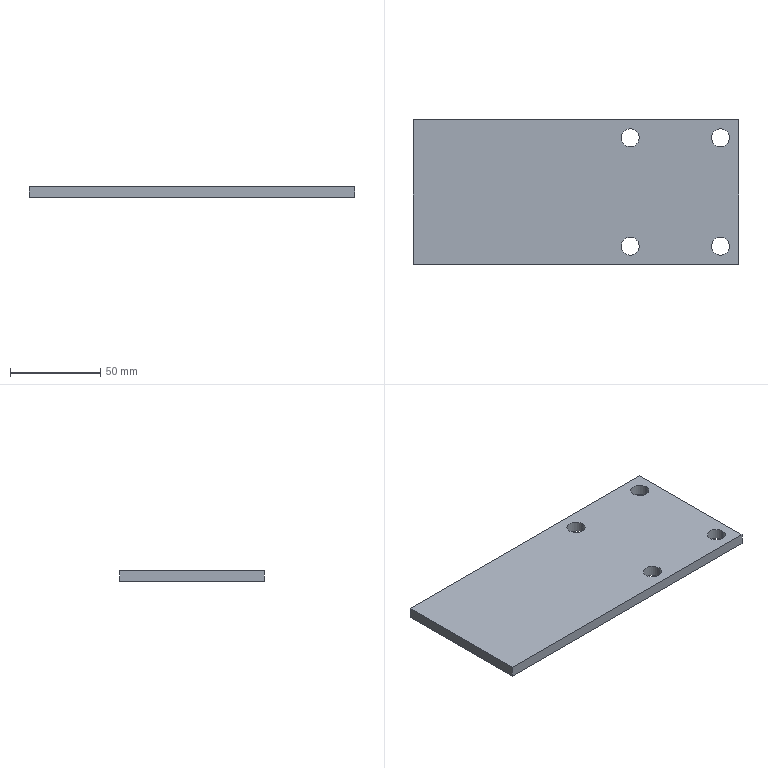Part | SolidWorks | features Extrusion 1, ICE 1 | 1 solid | 14 faces | box 180 x 80 x 6 mm | volume 84515 mm3 | cylinder 8 | plane 6 | commonest cylinder face diameters 10 x8
STEP:
#1=CARTESIAN_POINT('',(165.,9.999,0.));
#2=VERTEX_POINT('',#1);
#3=CARTESIAN_POINT('',(175.,9.999,0.));
#4=VERTEX_POINT('',#3);
#5=CARTESIAN_POINT('',(170.,9.999,0.));
#6=DIRECTION('',(0.,0.,1.));
#7=DIRECTION('',(1.,0.,0.));
#8=AXIS2_PLACEMENT_3D('',#5,#6,#7);
#9=CIRCLE('',#8,5.);
#10=EDGE_CURVE('',#2,#4,#9,.T.);
#11=ORIENTED_EDGE('',*,*,#10,.F.);
#12=CARTESIAN_POINT('',(165.,9.999,6.));
#13=VERTEX_POINT('',#12);
#14=CARTESIAN_POINT('',(165.,9.999,0.));
#15=DIRECTION('',(0.,0.,1.));
#16=VECTOR('',#15,1000.);
#17=LINE('',#14,#16);
#18=EDGE_CURVE('',#2,#13,#17,.T.);
#19=ORIENTED_EDGE('',*,*,#18,.T.);
#20=CARTESIAN_POINT('',(175.,9.999,6.));
#21=VERTEX_POINT('',#20);
#22=CARTESIAN_POINT('',(170.,9.999,6.));
#23=DIRECTION('',(0.,0.,1.));
#24=DIRECTION('',(1.,0.,0.));
#25=AXIS2_PLACEMENT_3D('',#22,#23,#24);
#26=CIRCLE('',#25,5.);
#27=EDGE_CURVE('',#13,#21,#26,.T.);
#28=ORIENTED_EDGE('',*,*,#27,.T.);
#29=CARTESIAN_POINT('',(175.,9.999,0.));
#30=DIRECTION('',(0.,0.,1.));
#31=VECTOR('',#30,1000.);
#32=LINE('',#29,#31);
#33=EDGE_CURVE('',#4,#21,#32,.T.);
#34=ORIENTED_EDGE('',*,*,#33,.F.);
#35=EDGE_LOOP('',(#11,#19,#28,#34));
#36=FACE_OUTER_BOUND('',#35,.T.);
#37=CARTESIAN_POINT('',(170.,9.999,0.));
#38=DIRECTION('',(0.,0.,1.));
#39=DIRECTION('',(1.,0.,0.));
#40=AXIS2_PLACEMENT_3D('',#37,#38,#39);
#41=CYLINDRICAL_SURFACE('',#40,5.);
#42=ADVANCED_FACE('',(#36),#41,.F.);
#43=CARTESIAN_POINT('',(115.,9.999,0.));
#44=VERTEX_POINT('',#43);
#45=CARTESIAN_POINT('',(125.,9.999,0.));
#46=VERTEX_POINT('',#45);
#47=CARTESIAN_POINT('',(120.,9.999,0.));
#48=DIRECTION('',(0.,0.,1.));
#49=DIRECTION('',(1.,0.,0.));
#50=AXIS2_PLACEMENT_3D('',#47,#48,#49);
#51=CIRCLE('',#50,5.);
#52=EDGE_CURVE('',#44,#46,#51,.T.);
#53=ORIENTED_EDGE('',*,*,#52,.F.);
#54=CARTESIAN_POINT('',(115.,9.999,6.));
#55=VERTEX_POINT('',#54);
#56=CARTESIAN_POINT('',(115.,9.999,0.));
#57=DIRECTION('',(0.,0.,1.));
#58=VECTOR('',#57,1000.);
#59=LINE('',#56,#58);
#60=EDGE_CURVE('',#44,#55,#59,.T.);
#61=ORIENTED_EDGE('',*,*,#60,.T.);
#62=CARTESIAN_POINT('',(125.,9.999,6.));
#63=VERTEX_POINT('',#62);
#64=CARTESIAN_POINT('',(120.,9.999,6.));
#65=DIRECTION('',(0.,0.,1.));
#66=DIRECTION('',(1.,0.,0.));
#67=AXIS2_PLACEMENT_3D('',#64,#65,#66);
#68=CIRCLE('',#67,5.);
#69=EDGE_CURVE('',#55,#63,#68,.T.);
#70=ORIENTED_EDGE('',*,*,#69,.T.);
#71=CARTESIAN_POINT('',(125.,9.999,0.));
#72=DIRECTION('',(0.,0.,1.));
#73=VECTOR('',#72,1000.);
#74=LINE('',#71,#73);
#75=EDGE_CURVE('',#46,#63,#74,.T.);
#76=ORIENTED_EDGE('',*,*,#75,.F.);
#77=EDGE_LOOP('',(#53,#61,#70,#76));
#78=FACE_OUTER_BOUND('',#77,.T.);
#79=CARTESIAN_POINT('',(120.,9.999,0.));
#80=DIRECTION('',(0.,0.,1.));
#81=DIRECTION('',(1.,0.,0.));
#82=AXIS2_PLACEMENT_3D('',#79,#80,#81);
#83=CYLINDRICAL_SURFACE('',#82,5.);
#84=ADVANCED_FACE('',(#78),#83,.F.);
#85=CARTESIAN_POINT('',(115.,69.999,0.));
#86=VERTEX_POINT('',#85);
#87=CARTESIAN_POINT('',(125.,69.999,0.));
#88=VERTEX_POINT('',#87);
#89=CARTESIAN_POINT('',(120.,69.999,0.));
#90=DIRECTION('',(0.,0.,1.));
#91=DIRECTION('',(1.,0.,0.));
#92=AXIS2_PLACEMENT_3D('',#89,#90,#91);
#93=CIRCLE('',#92,5.);
#94=EDGE_CURVE('',#86,#88,#93,.T.);
#95=ORIENTED_EDGE('',*,*,#94,.F.);
#96=CARTESIAN_POINT('',(115.,69.999,6.));
#97=VERTEX_POINT('',#96);
#98=CARTESIAN_POINT('',(115.,69.999,0.));
#99=DIRECTION('',(0.,0.,1.));
#100=VECTOR('',#99,1000.);
#101=LINE('',#98,#100);
#102=EDGE_CURVE('',#86,#97,#101,.T.);
#103=ORIENTED_EDGE('',*,*,#102,.T.);
#104=CARTESIAN_POINT('',(125.,69.999,6.));
#105=VERTEX_POINT('',#104);
#106=CARTESIAN_POINT('',(120.,69.999,6.));
#107=DIRECTION('',(0.,0.,1.));
#108=DIRECTION('',(1.,0.,0.));
#109=AXIS2_PLACEMENT_3D('',#106,#107,#108);
#110=CIRCLE('',#109,5.);
#111=EDGE_CURVE('',#97,#105,#110,.T.);
#112=ORIENTED_EDGE('',*,*,#111,.T.);
#113=CARTESIAN_POINT('',(125.,69.999,0.));
#114=DIRECTION('',(0.,0.,1.));
#115=VECTOR('',#114,1000.);
#116=LINE('',#113,#115);
#117=EDGE_CURVE('',#88,#105,#116,.T.);
#118=ORIENTED_EDGE('',*,*,#117,.F.);
#119=EDGE_LOOP('',(#95,#103,#112,#118));
#120=FACE_OUTER_BOUND('',#119,.T.);
#121=CARTESIAN_POINT('',(120.,69.999,0.));
#122=DIRECTION('',(0.,0.,1.));
#123=DIRECTION('',(1.,0.,0.));
#124=AXIS2_PLACEMENT_3D('',#121,#122,#123);
#125=CYLINDRICAL_SURFACE('',#124,5.);
#126=ADVANCED_FACE('',(#120),#125,.F.);
#127=CARTESIAN_POINT('',(165.,69.999,0.));
#128=VERTEX_POINT('',#127);
#129=CARTESIAN_POINT('',(175.,69.999,0.));
#130=VERTEX_POINT('',#129);
#131=CARTESIAN_POINT('',(170.,69.999,0.));
#132=DIRECTION('',(0.,0.,1.));
#133=DIRECTION('',(1.,0.,0.));
#134=AXIS2_PLACEMENT_3D('',#131,#132,#133);
#135=CIRCLE('',#134,5.);
#136=EDGE_CURVE('',#128,#130,#135,.T.);
#137=ORIENTED_EDGE('',*,*,#136,.F.);
#138=CARTESIAN_POINT('',(165.,69.999,6.));
#139=VERTEX_POINT('',#138);
#140=CARTESIAN_POINT('',(165.,69.999,0.));
#141=DIRECTION('',(0.,0.,1.));
#142=VECTOR('',#141,1000.);
#143=LINE('',#140,#142);
#144=EDGE_CURVE('',#128,#139,#143,.T.);
#145=ORIENTED_EDGE('',*,*,#144,.T.);
#146=CARTESIAN_POINT('',(175.,69.999,6.));
#147=VERTEX_POINT('',#146);
#148=CARTESIAN_POINT('',(170.,69.999,6.));
#149=DIRECTION('',(0.,0.,1.));
#150=DIRECTION('',(1.,0.,0.));
#151=AXIS2_PLACEMENT_3D('',#148,#149,#150);
#152=CIRCLE('',#151,5.);
#153=EDGE_CURVE('',#139,#147,#152,.T.);
#154=ORIENTED_EDGE('',*,*,#153,.T.);
#155=CARTESIAN_POINT('',(175.,69.999,0.));
#156=DIRECTION('',(0.,0.,1.));
#157=VECTOR('',#156,1000.);
#158=LINE('',#155,#157);
#159=EDGE_CURVE('',#130,#147,#158,.T.);
#160=ORIENTED_EDGE('',*,*,#159,.F.);
#161=EDGE_LOOP('',(#137,#145,#154,#160));
#162=FACE_OUTER_BOUND('',#161,.T.);
#163=CARTESIAN_POINT('',(170.,69.999,0.));
#164=DIRECTION('',(0.,0.,1.));
#165=DIRECTION('',(1.,0.,0.));
#166=AXIS2_PLACEMENT_3D('',#163,#164,#165);
#167=CYLINDRICAL_SURFACE('',#166,5.);
#168=ADVANCED_FACE('',(#162),#167,.F.);
#169=CARTESIAN_POINT('',(0.,0.,0.));
#170=VERTEX_POINT('',#169);
#171=CARTESIAN_POINT('',(180.,0.,0.));
#172=VERTEX_POINT('',#171);
#173=CARTESIAN_POINT('',(180.,0.,0.));
#174=DIRECTION('',(1.,0.,0.));
#175=VECTOR('',#174,1000.);
#176=LINE('',#173,#175);
#177=EDGE_CURVE('',#170,#172,#176,.T.);
#178=ORIENTED_EDGE('',*,*,#177,.T.);
#179=CARTESIAN_POINT('',(180.,0.,6.));
#180=VERTEX_POINT('',#179);
#181=CARTESIAN_POINT('',(180.,0.,6.));
#182=DIRECTION('',(0.,0.,-1.));
#183=VECTOR('',#182,1000.);
#184=LINE('',#181,#183);
#185=EDGE_CURVE('',#180,#172,#184,.T.);
#186=ORIENTED_EDGE('',*,*,#185,.F.);
#187=CARTESIAN_POINT('',(0.,0.,6.));
#188=VERTEX_POINT('',#187);
#189=CARTESIAN_POINT('',(180.,0.,6.));
#190=DIRECTION('',(1.,0.,0.));
#191=VECTOR('',#190,1000.);
#192=LINE('',#189,#191);
#193=EDGE_CURVE('',#188,#180,#192,.T.);
#194=ORIENTED_EDGE('',*,*,#193,.F.);
#195=CARTESIAN_POINT('',(0.,0.,6.));
#196=DIRECTION('',(0.,0.,-1.));
#197=VECTOR('',#196,1000.);
#198=LINE('',#195,#197);
#199=EDGE_CURVE('',#188,#170,#198,.T.);
#200=ORIENTED_EDGE('',*,*,#199,.T.);
#201=EDGE_LOOP('',(#178,#186,#194,#200));
#202=FACE_OUTER_BOUND('',#201,.T.);
#203=CARTESIAN_POINT('',(180.,0.,6.));
#204=DIRECTION('',(0.,1.,0.));
#205=DIRECTION('',(0.,0.,1.));
#206=AXIS2_PLACEMENT_3D('',#203,#204,#205);
#207=PLANE('',#206);
#208=ADVANCED_FACE('',(#202),#207,.F.);
#209=CARTESIAN_POINT('',(180.,80.,0.));
#210=VERTEX_POINT('',#209);
#211=CARTESIAN_POINT('',(180.,80.,0.));
#212=DIRECTION('',(0.,1.,0.));
#213=VECTOR('',#212,1000.);
#214=LINE('',#211,#213);
#215=EDGE_CURVE('',#172,#210,#214,.T.);
#216=ORIENTED_EDGE('',*,*,#215,.T.);
#217=CARTESIAN_POINT('',(180.,80.,6.));
#218=VERTEX_POINT('',#217);
#219=CARTESIAN_POINT('',(180.,80.,6.));
#220=DIRECTION('',(0.,0.,-1.));
#221=VECTOR('',#220,1000.);
#222=LINE('',#219,#221);
#223=EDGE_CURVE('',#218,#210,#222,.T.);
#224=ORIENTED_EDGE('',*,*,#223,.F.);
#225=CARTESIAN_POINT('',(180.,80.,6.));
#226=DIRECTION('',(0.,1.,0.));
#227=VECTOR('',#226,1000.);
#228=LINE('',#225,#227);
#229=EDGE_CURVE('',#180,#218,#228,.T.);
#230=ORIENTED_EDGE('',*,*,#229,.F.);
#231=ORIENTED_EDGE('',*,*,#185,.T.);
#232=EDGE_LOOP('',(#216,#224,#230,#231));
#233=FACE_OUTER_BOUND('',#232,.T.);
#234=CARTESIAN_POINT('',(180.,80.,6.));
#235=DIRECTION('',(-1.,0.,0.));
#236=DIRECTION('',(0.,0.,1.));
#237=AXIS2_PLACEMENT_3D('',#234,#235,#236);
#238=PLANE('',#237);
#239=ADVANCED_FACE('',(#233),#238,.F.);
#240=CARTESIAN_POINT('',(0.,80.,0.));
#241=VERTEX_POINT('',#240);
#242=CARTESIAN_POINT('',(0.,80.,0.));
#243=DIRECTION('',(-1.,0.,0.));
#244=VECTOR('',#243,1000.);
#245=LINE('',#242,#244);
#246=EDGE_CURVE('',#210,#241,#245,.T.);
#247=ORIENTED_EDGE('',*,*,#246,.T.);
#248=CARTESIAN_POINT('',(0.,80.,6.));
#249=VERTEX_POINT('',#248);
#250=CARTESIAN_POINT('',(0.,80.,6.));
#251=DIRECTION('',(0.,0.,-1.));
#252=VECTOR('',#251,1000.);
#253=LINE('',#250,#252);
#254=EDGE_CURVE('',#249,#241,#253,.T.);
#255=ORIENTED_EDGE('',*,*,#254,.F.);
#256=CARTESIAN_POINT('',(0.,80.,6.));
#257=DIRECTION('',(-1.,0.,0.));
#258=VECTOR('',#257,1000.);
#259=LINE('',#256,#258);
#260=EDGE_CURVE('',#218,#249,#259,.T.);
#261=ORIENTED_EDGE('',*,*,#260,.F.);
#262=ORIENTED_EDGE('',*,*,#223,.T.);
#263=EDGE_LOOP('',(#247,#255,#261,#262));
#264=FACE_OUTER_BOUND('',#263,.T.);
#265=CARTESIAN_POINT('',(0.,80.,6.));
#266=DIRECTION('',(0.,-1.,0.));
#267=DIRECTION('',(0.,0.,-1.));
#268=AXIS2_PLACEMENT_3D('',#265,#266,#267);
#269=PLANE('',#268);
#270=ADVANCED_FACE('',(#264),#269,.F.);
#271=CARTESIAN_POINT('',(0.,0.,0.));
#272=DIRECTION('',(0.,-1.,0.));
#273=VECTOR('',#272,1000.);
#274=LINE('',#271,#273);
#275=EDGE_CURVE('',#241,#170,#274,.T.);
#276=ORIENTED_EDGE('',*,*,#275,.T.);
#277=ORIENTED_EDGE('',*,*,#199,.F.);
#278=CARTESIAN_POINT('',(0.,0.,6.));
#279=DIRECTION('',(0.,-1.,0.));
#280=VECTOR('',#279,1000.);
#281=LINE('',#278,#280);
#282=EDGE_CURVE('',#249,#188,#281,.T.);
#283=ORIENTED_EDGE('',*,*,#282,.F.);
#284=ORIENTED_EDGE('',*,*,#254,.T.);
#285=EDGE_LOOP('',(#276,#277,#283,#284));
#286=FACE_OUTER_BOUND('',#285,.T.);
#287=CARTESIAN_POINT('',(0.,0.,6.));
#288=DIRECTION('',(1.,0.,0.));
#289=DIRECTION('',(0.,0.,-1.));
#290=AXIS2_PLACEMENT_3D('',#287,#288,#289);
#291=PLANE('',#290);
#292=ADVANCED_FACE('',(#286),#291,.F.);
#293=CARTESIAN_POINT('',(170.,9.999,6.));
#294=DIRECTION('',(0.,0.,1.));
#295=DIRECTION('',(1.,0.,0.));
#296=AXIS2_PLACEMENT_3D('',#293,#294,#295);
#297=CIRCLE('',#296,5.);
#298=EDGE_CURVE('',#21,#13,#297,.T.);
#299=ORIENTED_EDGE('',*,*,#298,.F.);
#300=ORIENTED_EDGE('',*,*,#27,.F.);
#301=EDGE_LOOP('',(#299,#300));
#302=FACE_BOUND('',#301,.T.);
#303=CARTESIAN_POINT('',(120.,9.999,6.));
#304=DIRECTION('',(0.,0.,1.));
#305=DIRECTION('',(1.,0.,0.));
#306=AXIS2_PLACEMENT_3D('',#303,#304,#305);
#307=CIRCLE('',#306,5.);
#308=EDGE_CURVE('',#63,#55,#307,.T.);
#309=ORIENTED_EDGE('',*,*,#308,.F.);
#310=ORIENTED_EDGE('',*,*,#69,.F.);
#311=EDGE_LOOP('',(#309,#310));
#312=FACE_BOUND('',#311,.T.);
#313=CARTESIAN_POINT('',(120.,69.999,6.));
#314=DIRECTION('',(0.,0.,1.));
#315=DIRECTION('',(1.,0.,0.));
#316=AXIS2_PLACEMENT_3D('',#313,#314,#315);
#317=CIRCLE('',#316,5.);
#318=EDGE_CURVE('',#105,#97,#317,.T.);
#319=ORIENTED_EDGE('',*,*,#318,.F.);
#320=ORIENTED_EDGE('',*,*,#111,.F.);
#321=EDGE_LOOP('',(#319,#320));
#322=FACE_BOUND('',#321,.T.);
#323=CARTESIAN_POINT('',(170.,69.999,6.));
#324=DIRECTION('',(0.,0.,1.));
#325=DIRECTION('',(1.,0.,0.));
#326=AXIS2_PLACEMENT_3D('',#323,#324,#325);
#327=CIRCLE('',#326,5.);
#328=EDGE_CURVE('',#147,#139,#327,.T.);
#329=ORIENTED_EDGE('',*,*,#328,.F.);
#330=ORIENTED_EDGE('',*,*,#153,.F.);
#331=EDGE_LOOP('',(#329,#330));
#332=FACE_BOUND('',#331,.T.);
#333=ORIENTED_EDGE('',*,*,#193,.T.);
#334=ORIENTED_EDGE('',*,*,#229,.T.);
#335=ORIENTED_EDGE('',*,*,#260,.T.);
#336=ORIENTED_EDGE('',*,*,#282,.T.);
#337=EDGE_LOOP('',(#333,#334,#335,#336));
#338=FACE_OUTER_BOUND('',#337,.T.);
#339=CARTESIAN_POINT('',(0.,0.,6.));
#340=DIRECTION('',(0.,0.,-1.));
#341=DIRECTION('',(-1.,0.,0.));
#342=AXIS2_PLACEMENT_3D('',#339,#340,#341);
#343=PLANE('',#342);
#344=ADVANCED_FACE('',(#302,#312,#322,#332,#338),#343,.F.);
#345=CARTESIAN_POINT('',(170.,9.999,0.));
#346=DIRECTION('',(0.,0.,1.));
#347=DIRECTION('',(1.,0.,0.));
#348=AXIS2_PLACEMENT_3D('',#345,#346,#347);
#349=CIRCLE('',#348,5.);
#350=EDGE_CURVE('',#4,#2,#349,.T.);
#351=ORIENTED_EDGE('',*,*,#350,.T.);
#352=ORIENTED_EDGE('',*,*,#10,.T.);
#353=EDGE_LOOP('',(#351,#352));
#354=FACE_BOUND('',#353,.T.);
#355=CARTESIAN_POINT('',(120.,9.999,0.));
#356=DIRECTION('',(0.,0.,1.));
#357=DIRECTION('',(1.,0.,0.));
#358=AXIS2_PLACEMENT_3D('',#355,#356,#357);
#359=CIRCLE('',#358,5.);
#360=EDGE_CURVE('',#46,#44,#359,.T.);
#361=ORIENTED_EDGE('',*,*,#360,.T.);
#362=ORIENTED_EDGE('',*,*,#52,.T.);
#363=EDGE_LOOP('',(#361,#362));
#364=FACE_BOUND('',#363,.T.);
#365=CARTESIAN_POINT('',(120.,69.999,0.));
#366=DIRECTION('',(0.,0.,1.));
#367=DIRECTION('',(1.,0.,0.));
#368=AXIS2_PLACEMENT_3D('',#365,#366,#367);
#369=CIRCLE('',#368,5.);
#370=EDGE_CURVE('',#88,#86,#369,.T.);
#371=ORIENTED_EDGE('',*,*,#370,.T.);
#372=ORIENTED_EDGE('',*,*,#94,.T.);
#373=EDGE_LOOP('',(#371,#372));
#374=FACE_BOUND('',#373,.T.);
#375=CARTESIAN_POINT('',(170.,69.999,0.));
#376=DIRECTION('',(0.,0.,1.));
#377=DIRECTION('',(1.,0.,0.));
#378=AXIS2_PLACEMENT_3D('',#375,#376,#377);
#379=CIRCLE('',#378,5.);
#380=EDGE_CURVE('',#130,#128,#379,.T.);
#381=ORIENTED_EDGE('',*,*,#380,.T.);
#382=ORIENTED_EDGE('',*,*,#136,.T.);
#383=EDGE_LOOP('',(#381,#382));
#384=FACE_BOUND('',#383,.T.);
#385=ORIENTED_EDGE('',*,*,#177,.F.);
#386=ORIENTED_EDGE('',*,*,#275,.F.);
#387=ORIENTED_EDGE('',*,*,#246,.F.);
#388=ORIENTED_EDGE('',*,*,#215,.F.);
#389=EDGE_LOOP('',(#385,#386,#387,#388));
#390=FACE_OUTER_BOUND('',#389,.T.);
#391=CARTESIAN_POINT('',(0.,0.,0.));
#392=DIRECTION('',(0.,0.,-1.));
#393=DIRECTION('',(-1.,0.,0.));
#394=AXIS2_PLACEMENT_3D('',#391,#392,#393);
#395=PLANE('',#394);
#396=ADVANCED_FACE('',(#354,#364,#374,#384,#390),#395,.T.);
#397=ORIENTED_EDGE('',*,*,#144,.F.);
#398=ORIENTED_EDGE('',*,*,#380,.F.);
#399=ORIENTED_EDGE('',*,*,#159,.T.);
#400=ORIENTED_EDGE('',*,*,#328,.T.);
#401=EDGE_LOOP('',(#397,#398,#399,#400));
#402=FACE_OUTER_BOUND('',#401,.T.);
#403=CARTESIAN_POINT('',(170.,69.999,0.));
#404=DIRECTION('',(0.,0.,1.));
#405=DIRECTION('',(1.,0.,0.));
#406=AXIS2_PLACEMENT_3D('',#403,#404,#405);
#407=CYLINDRICAL_SURFACE('',#406,5.);
#408=ADVANCED_FACE('',(#402),#407,.F.);
#409=ORIENTED_EDGE('',*,*,#102,.F.);
#410=ORIENTED_EDGE('',*,*,#370,.F.);
#411=ORIENTED_EDGE('',*,*,#117,.T.);
#412=ORIENTED_EDGE('',*,*,#318,.T.);
#413=EDGE_LOOP('',(#409,#410,#411,#412));
#414=FACE_OUTER_BOUND('',#413,.T.);
#415=CARTESIAN_POINT('',(120.,69.999,0.));
#416=DIRECTION('',(0.,0.,1.));
#417=DIRECTION('',(1.,0.,0.));
#418=AXIS2_PLACEMENT_3D('',#415,#416,#417);
#419=CYLINDRICAL_SURFACE('',#418,5.);
#420=ADVANCED_FACE('',(#414),#419,.F.);
#421=ORIENTED_EDGE('',*,*,#60,.F.);
#422=ORIENTED_EDGE('',*,*,#360,.F.);
#423=ORIENTED_EDGE('',*,*,#75,.T.);
#424=ORIENTED_EDGE('',*,*,#308,.T.);
#425=EDGE_LOOP('',(#421,#422,#423,#424));
#426=FACE_OUTER_BOUND('',#425,.T.);
#427=CARTESIAN_POINT('',(120.,9.999,0.));
#428=DIRECTION('',(0.,0.,1.));
#429=DIRECTION('',(1.,0.,0.));
#430=AXIS2_PLACEMENT_3D('',#427,#428,#429);
#431=CYLINDRICAL_SURFACE('',#430,5.);
#432=ADVANCED_FACE('',(#426),#431,.F.);
#433=ORIENTED_EDGE('',*,*,#18,.F.);
#434=ORIENTED_EDGE('',*,*,#350,.F.);
#435=ORIENTED_EDGE('',*,*,#33,.T.);
#436=ORIENTED_EDGE('',*,*,#298,.T.);
#437=EDGE_LOOP('',(#433,#434,#435,#436));
#438=FACE_OUTER_BOUND('',#437,.T.);
#439=CARTESIAN_POINT('',(170.,9.999,0.));
#440=DIRECTION('',(0.,0.,1.));
#441=DIRECTION('',(1.,0.,0.));
#442=AXIS2_PLACEMENT_3D('',#439,#440,#441);
#443=CYLINDRICAL_SURFACE('',#442,5.);
#444=ADVANCED_FACE('',(#438),#443,.F.);
#445=CLOSED_SHELL('',(#42,#84,#126,#168,#208,#239,#270,#292,#344,#396,#408,#420,#432,#444));
#446=MANIFOLD_SOLID_BREP('',#445);
#447=CARTESIAN_POINT('',(0.,0.,0.));
#448=DIRECTION('',(0.,0.,1.));
#449=DIRECTION('',(1.,0.,0.));
#450=AXIS2_PLACEMENT_3D('',#447,#448,#449);
#451=(LENGTH_UNIT()NAMED_UNIT(*)SI_UNIT(.MILLI.,.METRE.));
#452=UNCERTAINTY_MEASURE_WITH_UNIT(LENGTH_MEASURE(0.00001),#451,'','');
#453=(NAMED_UNIT(*)PLANE_ANGLE_UNIT()SI_UNIT($,.RADIAN.));
#454=(NAMED_UNIT(*)SI_UNIT($,.STERADIAN.)SOLID_ANGLE_UNIT());
#455=(GEOMETRIC_REPRESENTATION_CONTEXT(3)GLOBAL_UNCERTAINTY_ASSIGNED_CONTEXT((#452))GLOBAL_UNIT_ASSIGNED_CONTEXT((#451,#453,#454))REPRESENTATION_CONTEXT('',''));
#456=ADVANCED_BREP_SHAPE_REPRESENTATION('',(#446,#450),#455);